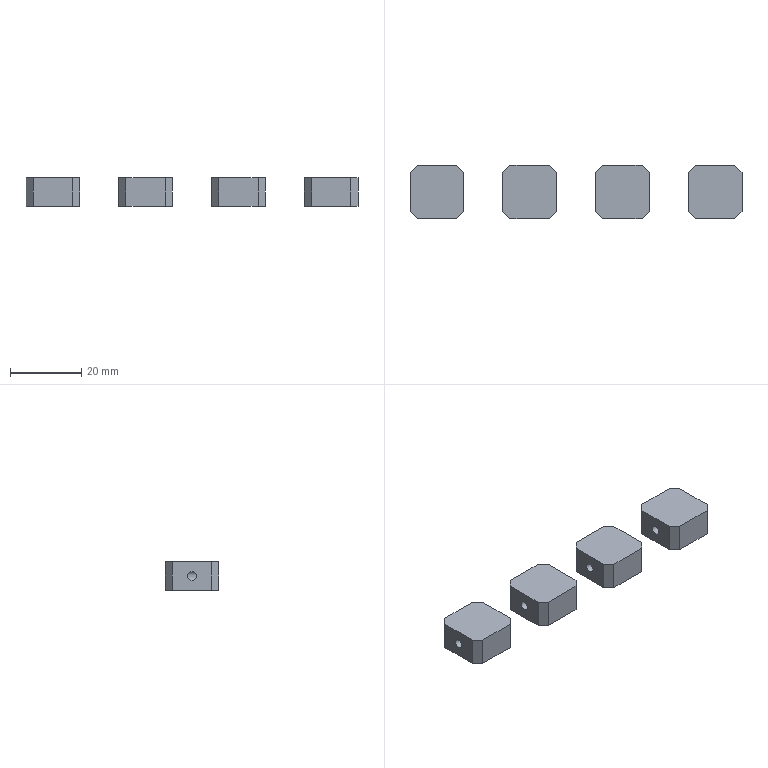Part | 4 solids | 52 faces | box 93 x 15 x 8 mm | volume 6470 mm3 | plane 40 | cylinder 8 | cone 4 | commonest cylinder face diameters 2.5 x4 3.3 x4
STEP:
#1=CARTESIAN_POINT('',(-5.5,7.5,8.));
#2=VERTEX_POINT('',#1);
#3=CARTESIAN_POINT('',(-7.5,5.5,8.));
#4=VERTEX_POINT('',#3);
#5=CARTESIAN_POINT('',(-6.5,6.5,8.));
#6=DIRECTION('',(-0.7071,-0.7071,0.));
#7=VECTOR('',#6,1000.);
#8=LINE('',#5,#7);
#9=EDGE_CURVE('',#2,#4,#8,.T.);
#10=ORIENTED_EDGE('',*,*,#9,.F.);
#11=CARTESIAN_POINT('',(-5.5,7.5,0.));
#12=VERTEX_POINT('',#11);
#13=CARTESIAN_POINT('',(-5.5,7.5,8.));
#14=DIRECTION('',(0.,0.,1.));
#15=VECTOR('',#14,1000.);
#16=LINE('',#13,#15);
#17=EDGE_CURVE('',#12,#2,#16,.T.);
#18=ORIENTED_EDGE('',*,*,#17,.F.);
#19=CARTESIAN_POINT('',(-7.5,5.5,0.));
#20=VERTEX_POINT('',#19);
#21=CARTESIAN_POINT('',(-7.5,5.5,0.));
#22=DIRECTION('',(0.7071,0.7071,0.));
#23=VECTOR('',#22,1000.);
#24=LINE('',#21,#23);
#25=EDGE_CURVE('',#20,#12,#24,.T.);
#26=ORIENTED_EDGE('',*,*,#25,.F.);
#27=CARTESIAN_POINT('',(-7.5,5.5,8.));
#28=DIRECTION('',(0.,0.,-1.));
#29=VECTOR('',#28,1000.);
#30=LINE('',#27,#29);
#31=EDGE_CURVE('',#4,#20,#30,.T.);
#32=ORIENTED_EDGE('',*,*,#31,.F.);
#33=EDGE_LOOP('',(#10,#18,#26,#32));
#34=FACE_BOUND('',#33,.T.);
#35=CARTESIAN_POINT('',(-7.5,5.5,8.));
#36=DIRECTION('',(0.7071,-0.7071,0.));
#37=DIRECTION('',(0.,0.,-1.));
#38=AXIS2_PLACEMENT_3D('',#35,#36,#37);
#39=PLANE('',#38);
#40=ADVANCED_FACE('',(#34),#39,.F.);
#41=CARTESIAN_POINT('',(-7.5,-5.5,8.));
#42=VERTEX_POINT('',#41);
#43=CARTESIAN_POINT('',(-5.5,-7.5,8.));
#44=VERTEX_POINT('',#43);
#45=CARTESIAN_POINT('',(-6.5,-6.5,8.));
#46=DIRECTION('',(0.7071,-0.7071,0.));
#47=VECTOR('',#46,1000.);
#48=LINE('',#45,#47);
#49=EDGE_CURVE('',#42,#44,#48,.T.);
#50=ORIENTED_EDGE('',*,*,#49,.F.);
#51=CARTESIAN_POINT('',(-7.5,-5.5,0.));
#52=VERTEX_POINT('',#51);
#53=CARTESIAN_POINT('',(-7.5,-5.5,8.));
#54=DIRECTION('',(0.,0.,1.));
#55=VECTOR('',#54,1000.);
#56=LINE('',#53,#55);
#57=EDGE_CURVE('',#52,#42,#56,.T.);
#58=ORIENTED_EDGE('',*,*,#57,.F.);
#59=CARTESIAN_POINT('',(-5.5,-7.5,0.));
#60=VERTEX_POINT('',#59);
#61=CARTESIAN_POINT('',(-5.5,-7.5,0.));
#62=DIRECTION('',(-0.7071,0.7071,0.));
#63=VECTOR('',#62,1000.);
#64=LINE('',#61,#63);
#65=EDGE_CURVE('',#60,#52,#64,.T.);
#66=ORIENTED_EDGE('',*,*,#65,.F.);
#67=CARTESIAN_POINT('',(-5.5,-7.5,8.));
#68=DIRECTION('',(0.,0.,-1.));
#69=VECTOR('',#68,1000.);
#70=LINE('',#67,#69);
#71=EDGE_CURVE('',#44,#60,#70,.T.);
#72=ORIENTED_EDGE('',*,*,#71,.F.);
#73=EDGE_LOOP('',(#50,#58,#66,#72));
#74=FACE_BOUND('',#73,.T.);
#75=CARTESIAN_POINT('',(-5.5,-7.5,8.));
#76=DIRECTION('',(0.7071,0.7071,0.));
#77=DIRECTION('',(0.,0.,-1.));
#78=AXIS2_PLACEMENT_3D('',#75,#76,#77);
#79=PLANE('',#78);
#80=ADVANCED_FACE('',(#74),#79,.F.);
#81=CARTESIAN_POINT('',(5.5,-7.5,8.));
#82=VERTEX_POINT('',#81);
#83=CARTESIAN_POINT('',(7.5,-5.5,8.));
#84=VERTEX_POINT('',#83);
#85=CARTESIAN_POINT('',(6.5,-6.5,8.));
#86=DIRECTION('',(0.7071,0.7071,0.));
#87=VECTOR('',#86,1000.);
#88=LINE('',#85,#87);
#89=EDGE_CURVE('',#82,#84,#88,.T.);
#90=ORIENTED_EDGE('',*,*,#89,.F.);
#91=CARTESIAN_POINT('',(5.5,-7.5,0.));
#92=VERTEX_POINT('',#91);
#93=CARTESIAN_POINT('',(5.5,-7.5,8.));
#94=DIRECTION('',(0.,0.,1.));
#95=VECTOR('',#94,1000.);
#96=LINE('',#93,#95);
#97=EDGE_CURVE('',#92,#82,#96,.T.);
#98=ORIENTED_EDGE('',*,*,#97,.F.);
#99=CARTESIAN_POINT('',(7.5,-5.5,0.));
#100=VERTEX_POINT('',#99);
#101=CARTESIAN_POINT('',(7.5,-5.5,0.));
#102=DIRECTION('',(-0.7071,-0.7071,0.));
#103=VECTOR('',#102,1000.);
#104=LINE('',#101,#103);
#105=EDGE_CURVE('',#100,#92,#104,.T.);
#106=ORIENTED_EDGE('',*,*,#105,.F.);
#107=CARTESIAN_POINT('',(7.5,-5.5,8.));
#108=DIRECTION('',(0.,0.,-1.));
#109=VECTOR('',#108,1000.);
#110=LINE('',#107,#109);
#111=EDGE_CURVE('',#84,#100,#110,.T.);
#112=ORIENTED_EDGE('',*,*,#111,.F.);
#113=EDGE_LOOP('',(#90,#98,#106,#112));
#114=FACE_BOUND('',#113,.T.);
#115=CARTESIAN_POINT('',(7.5,-5.5,8.));
#116=DIRECTION('',(-0.7071,0.7071,0.));
#117=DIRECTION('',(0.,0.,-1.));
#118=AXIS2_PLACEMENT_3D('',#115,#116,#117);
#119=PLANE('',#118);
#120=ADVANCED_FACE('',(#114),#119,.F.);
#121=CARTESIAN_POINT('',(7.5,5.5,8.));
#122=VERTEX_POINT('',#121);
#123=CARTESIAN_POINT('',(5.5,7.5,8.));
#124=VERTEX_POINT('',#123);
#125=CARTESIAN_POINT('',(6.5,6.5,8.));
#126=DIRECTION('',(-0.7071,0.7071,0.));
#127=VECTOR('',#126,1000.);
#128=LINE('',#125,#127);
#129=EDGE_CURVE('',#122,#124,#128,.T.);
#130=ORIENTED_EDGE('',*,*,#129,.F.);
#131=CARTESIAN_POINT('',(7.5,5.5,0.));
#132=VERTEX_POINT('',#131);
#133=CARTESIAN_POINT('',(7.5,5.5,8.));
#134=DIRECTION('',(0.,0.,1.));
#135=VECTOR('',#134,1000.);
#136=LINE('',#133,#135);
#137=EDGE_CURVE('',#132,#122,#136,.T.);
#138=ORIENTED_EDGE('',*,*,#137,.F.);
#139=CARTESIAN_POINT('',(5.5,7.5,0.));
#140=VERTEX_POINT('',#139);
#141=CARTESIAN_POINT('',(5.5,7.5,0.));
#142=DIRECTION('',(0.7071,-0.7071,0.));
#143=VECTOR('',#142,1000.);
#144=LINE('',#141,#143);
#145=EDGE_CURVE('',#140,#132,#144,.T.);
#146=ORIENTED_EDGE('',*,*,#145,.F.);
#147=CARTESIAN_POINT('',(5.5,7.5,8.));
#148=DIRECTION('',(0.,0.,-1.));
#149=VECTOR('',#148,1000.);
#150=LINE('',#147,#149);
#151=EDGE_CURVE('',#124,#140,#150,.T.);
#152=ORIENTED_EDGE('',*,*,#151,.F.);
#153=EDGE_LOOP('',(#130,#138,#146,#152));
#154=FACE_BOUND('',#153,.T.);
#155=CARTESIAN_POINT('',(5.5,7.5,8.));
#156=DIRECTION('',(-0.7071,-0.7071,0.));
#157=DIRECTION('',(0.,0.,-1.));
#158=AXIS2_PLACEMENT_3D('',#155,#156,#157);
#159=PLANE('',#158);
#160=ADVANCED_FACE('',(#154),#159,.F.);
#161=CARTESIAN_POINT('',(-7.5,7.5,0.));
#162=DIRECTION('',(-1.,0.,0.));
#163=VECTOR('',#162,1000.);
#164=LINE('',#161,#163);
#165=EDGE_CURVE('',#140,#12,#164,.T.);
#166=ORIENTED_EDGE('',*,*,#165,.F.);
#167=ORIENTED_EDGE('',*,*,#145,.T.);
#168=CARTESIAN_POINT('',(7.5,7.5,0.));
#169=DIRECTION('',(0.,1.,0.));
#170=VECTOR('',#169,1000.);
#171=LINE('',#168,#170);
#172=EDGE_CURVE('',#100,#132,#171,.T.);
#173=ORIENTED_EDGE('',*,*,#172,.F.);
#174=ORIENTED_EDGE('',*,*,#105,.T.);
#175=CARTESIAN_POINT('',(-7.5,-7.5,0.));
#176=DIRECTION('',(1.,0.,0.));
#177=VECTOR('',#176,1000.);
#178=LINE('',#175,#177);
#179=EDGE_CURVE('',#60,#92,#178,.T.);
#180=ORIENTED_EDGE('',*,*,#179,.F.);
#181=ORIENTED_EDGE('',*,*,#65,.T.);
#182=CARTESIAN_POINT('',(-7.5,7.5,0.));
#183=DIRECTION('',(0.,-1.,0.));
#184=VECTOR('',#183,1000.);
#185=LINE('',#182,#184);
#186=EDGE_CURVE('',#20,#52,#185,.T.);
#187=ORIENTED_EDGE('',*,*,#186,.F.);
#188=ORIENTED_EDGE('',*,*,#25,.T.);
#189=EDGE_LOOP('',(#166,#167,#173,#174,#180,#181,#187,#188));
#190=FACE_BOUND('',#189,.T.);
#191=CARTESIAN_POINT('',(0.,0.,0.));
#192=DIRECTION('',(0.,0.,1.));
#193=DIRECTION('',(1.,0.,0.));
#194=AXIS2_PLACEMENT_3D('',#191,#192,#193);
#195=PLANE('',#194);
#196=ADVANCED_FACE('',(#190),#195,.F.);
#197=CARTESIAN_POINT('',(7.5,7.5,8.));
#198=DIRECTION('',(0.,1.,0.));
#199=VECTOR('',#198,1000.);
#200=LINE('',#197,#199);
#201=EDGE_CURVE('',#84,#122,#200,.T.);
#202=ORIENTED_EDGE('',*,*,#201,.T.);
#203=ORIENTED_EDGE('',*,*,#129,.T.);
#204=CARTESIAN_POINT('',(-7.5,7.5,8.));
#205=DIRECTION('',(-1.,0.,0.));
#206=VECTOR('',#205,1000.);
#207=LINE('',#204,#206);
#208=EDGE_CURVE('',#124,#2,#207,.T.);
#209=ORIENTED_EDGE('',*,*,#208,.T.);
#210=ORIENTED_EDGE('',*,*,#9,.T.);
#211=CARTESIAN_POINT('',(-7.5,7.5,8.));
#212=DIRECTION('',(0.,-1.,0.));
#213=VECTOR('',#212,1000.);
#214=LINE('',#211,#213);
#215=EDGE_CURVE('',#4,#42,#214,.T.);
#216=ORIENTED_EDGE('',*,*,#215,.T.);
#217=ORIENTED_EDGE('',*,*,#49,.T.);
#218=CARTESIAN_POINT('',(-7.5,-7.5,8.));
#219=DIRECTION('',(1.,0.,0.));
#220=VECTOR('',#219,1000.);
#221=LINE('',#218,#220);
#222=EDGE_CURVE('',#44,#82,#221,.T.);
#223=ORIENTED_EDGE('',*,*,#222,.T.);
#224=ORIENTED_EDGE('',*,*,#89,.T.);
#225=EDGE_LOOP('',(#202,#203,#209,#210,#216,#217,#223,#224));
#226=FACE_BOUND('',#225,.T.);
#227=CARTESIAN_POINT('',(0.,0.,8.));
#228=DIRECTION('',(0.,0.,1.));
#229=DIRECTION('',(1.,0.,0.));
#230=AXIS2_PLACEMENT_3D('',#227,#228,#229);
#231=PLANE('',#230);
#232=ADVANCED_FACE('',(#226),#231,.T.);
#233=ORIENTED_EDGE('',*,*,#179,.T.);
#234=ORIENTED_EDGE('',*,*,#97,.T.);
#235=ORIENTED_EDGE('',*,*,#222,.F.);
#236=ORIENTED_EDGE('',*,*,#71,.T.);
#237=EDGE_LOOP('',(#233,#234,#235,#236));
#238=FACE_BOUND('',#237,.T.);
#239=CARTESIAN_POINT('',(-7.5,-7.5,8.));
#240=DIRECTION('',(0.,1.,0.));
#241=DIRECTION('',(0.,0.,1.));
#242=AXIS2_PLACEMENT_3D('',#239,#240,#241);
#243=PLANE('',#242);
#244=ADVANCED_FACE('',(#238),#243,.F.);
#245=ORIENTED_EDGE('',*,*,#186,.T.);
#246=ORIENTED_EDGE('',*,*,#57,.T.);
#247=ORIENTED_EDGE('',*,*,#215,.F.);
#248=ORIENTED_EDGE('',*,*,#31,.T.);
#249=EDGE_LOOP('',(#245,#246,#247,#248));
#250=FACE_BOUND('',#249,.T.);
#251=CARTESIAN_POINT('',(-7.5,0.,5.25));
#252=VERTEX_POINT('',#251);
#253=CARTESIAN_POINT('',(-7.5,0.,4.));
#254=DIRECTION('',(-1.,0.,0.));
#255=DIRECTION('',(0.,0.,1.));
#256=AXIS2_PLACEMENT_3D('',#253,#254,#255);
#257=CIRCLE('',#256,1.25);
#258=EDGE_CURVE('',#252,#252,#257,.T.);
#259=ORIENTED_EDGE('',*,*,#258,.F.);
#260=EDGE_LOOP('',(#259));
#261=FACE_BOUND('',#260,.T.);
#262=CARTESIAN_POINT('',(-7.5,7.5,8.));
#263=DIRECTION('',(1.,0.,0.));
#264=DIRECTION('',(0.,1.,0.));
#265=AXIS2_PLACEMENT_3D('',#262,#263,#264);
#266=PLANE('',#265);
#267=ADVANCED_FACE('',(#250,#261),#266,.F.);
#268=ORIENTED_EDGE('',*,*,#208,.F.);
#269=ORIENTED_EDGE('',*,*,#151,.T.);
#270=ORIENTED_EDGE('',*,*,#165,.T.);
#271=ORIENTED_EDGE('',*,*,#17,.T.);
#272=EDGE_LOOP('',(#268,#269,#270,#271));
#273=FACE_BOUND('',#272,.T.);
#274=CARTESIAN_POINT('',(0.,7.5,5.65));
#275=VERTEX_POINT('',#274);
#276=CARTESIAN_POINT('',(0.,7.5,4.));
#277=DIRECTION('',(0.,1.,0.));
#278=DIRECTION('',(0.,0.,1.));
#279=AXIS2_PLACEMENT_3D('',#276,#277,#278);
#280=CIRCLE('',#279,1.65);
#281=EDGE_CURVE('',#275,#275,#280,.T.);
#282=ORIENTED_EDGE('',*,*,#281,.F.);
#283=EDGE_LOOP('',(#282));
#284=FACE_BOUND('',#283,.T.);
#285=CARTESIAN_POINT('',(-7.5,7.5,8.));
#286=DIRECTION('',(0.,-1.,0.));
#287=DIRECTION('',(0.,0.,-1.));
#288=AXIS2_PLACEMENT_3D('',#285,#286,#287);
#289=PLANE('',#288);
#290=ADVANCED_FACE('',(#273,#284),#289,.F.);
#291=ORIENTED_EDGE('',*,*,#172,.T.);
#292=ORIENTED_EDGE('',*,*,#137,.T.);
#293=ORIENTED_EDGE('',*,*,#201,.F.);
#294=ORIENTED_EDGE('',*,*,#111,.T.);
#295=EDGE_LOOP('',(#291,#292,#293,#294));
#296=FACE_BOUND('',#295,.T.);
#297=CARTESIAN_POINT('',(7.5,7.5,8.));
#298=DIRECTION('',(-1.,0.,0.));
#299=DIRECTION('',(0.,-1.,0.));
#300=AXIS2_PLACEMENT_3D('',#297,#298,#299);
#301=PLANE('',#300);
#302=ADVANCED_FACE('',(#296),#301,.F.);
#303=CARTESIAN_POINT('',(0.,-2.6,5.65));
#304=VERTEX_POINT('',#303);
#305=CARTESIAN_POINT('',(0.,-2.6,4.));
#306=DIRECTION('',(0.,1.,0.));
#307=DIRECTION('',(0.,0.,1.));
#308=AXIS2_PLACEMENT_3D('',#305,#306,#307);
#309=CIRCLE('',#308,1.65);
#310=EDGE_CURVE('',#304,#304,#309,.T.);
#311=ORIENTED_EDGE('',*,*,#310,.T.);
#312=EDGE_LOOP('',(#311));
#313=FACE_BOUND('',#312,.T.);
#314=CARTESIAN_POINT('',(0.,-3.591,4.));
#315=VERTEX_POINT('',#314);
#316=VERTEX_LOOP('',#315);
#317=FACE_BOUND('',#316,.T.);
#318=CARTESIAN_POINT('',(0.,-2.6,4.));
#319=DIRECTION('',(0.,1.,0.));
#320=DIRECTION('',(0.,0.,1.));
#321=AXIS2_PLACEMENT_3D('',#318,#319,#320);
#322=CONICAL_SURFACE('',#321,1.65,1.03);
#323=ADVANCED_FACE('',(#313,#317),#322,.F.);
#324=ORIENTED_EDGE('',*,*,#310,.F.);
#325=EDGE_LOOP('',(#324));
#326=FACE_BOUND('',#325,.T.);
#327=ORIENTED_EDGE('',*,*,#281,.T.);
#328=EDGE_LOOP('',(#327));
#329=FACE_BOUND('',#328,.T.);
#330=CARTESIAN_POINT('',(-1.077,0.,2.75));
#331=VERTEX_POINT('',#330);
#332=CARTESIAN_POINT('',(-1.417,0.9718,3.012));
#333=CARTESIAN_POINT('',(-0.9074,-0.0006623,2.619));
#334=CARTESIAN_POINT('',(-1.416,-0.9692,3.011));
#335=CARTESIAN_POINT('',(-1.767,-1.39,3.997));
#336=CARTESIAN_POINT('',(-1.416,-0.9715,4.989));
#337=CARTESIAN_POINT('',(-0.9074,0.00335,5.381));
#338=CARTESIAN_POINT('',(-1.416,0.9694,4.988));
#339=CARTESIAN_POINT('',(-1.767,1.39,4.003));
#340=CARTESIAN_POINT('',(-1.417,0.9718,3.012));
#341=CARTESIAN_POINT('',(-0.9074,-0.0006623,2.619));
#342=CARTESIAN_POINT('',(-1.416,-0.9692,3.011));
#343=B_SPLINE_CURVE_WITH_KNOTS('',3,(#332,#333,#334,#335,#336,#337,#338,#339,#340,#341,#342),.UNSPECIFIED.,.T.,.F.,(1,1,1,1,1,1,1,1,1,1,1,1,1,1,1),(-0.003071,-0.002047,-0.001024,0.,0.001024,0.002047,0.003071,0.004095,0.005119,0.006142,0.007166,0.00819,0.009214,0.01024,0.01126),.UNSPECIFIED.);
#344=EDGE_CURVE('',#331,#331,#343,.T.);
#345=ORIENTED_EDGE('',*,*,#344,.T.);
#346=EDGE_LOOP('',(#345));
#347=FACE_BOUND('',#346,.T.);
#348=CARTESIAN_POINT('',(0.,7.5,4.));
#349=DIRECTION('',(0.,1.,0.));
#350=DIRECTION('',(0.,0.,1.));
#351=AXIS2_PLACEMENT_3D('',#348,#349,#350);
#352=CYLINDRICAL_SURFACE('',#351,1.65);
#353=ADVANCED_FACE('',(#326,#329,#347),#352,.F.);
#354=ORIENTED_EDGE('',*,*,#344,.F.);
#355=EDGE_LOOP('',(#354));
#356=FACE_BOUND('',#355,.T.);
#357=ORIENTED_EDGE('',*,*,#258,.T.);
#358=EDGE_LOOP('',(#357));
#359=FACE_BOUND('',#358,.T.);
#360=CARTESIAN_POINT('',(-7.5,0.,4.));
#361=DIRECTION('',(-1.,0.,0.));
#362=DIRECTION('',(0.,0.,1.));
#363=AXIS2_PLACEMENT_3D('',#360,#361,#362);
#364=CYLINDRICAL_SURFACE('',#363,1.25);
#365=ADVANCED_FACE('',(#356,#359),#364,.F.);
#366=CLOSED_SHELL('',(#40,#80,#120,#160,#196,#232,#244,#267,#290,#302,#323,#353,#365));
#367=MANIFOLD_SOLID_BREP('',#366);
#368=CARTESIAN_POINT('',(20.5,7.5,8.));
#369=VERTEX_POINT('',#368);
#370=CARTESIAN_POINT('',(18.5,5.5,8.));
#371=VERTEX_POINT('',#370);
#372=CARTESIAN_POINT('',(19.5,6.5,8.));
#373=DIRECTION('',(-0.7071,-0.7071,0.));
#374=VECTOR('',#373,1000.);
#375=LINE('',#372,#374);
#376=EDGE_CURVE('',#369,#371,#375,.T.);
#377=ORIENTED_EDGE('',*,*,#376,.F.);
#378=CARTESIAN_POINT('',(20.5,7.5,0.));
#379=VERTEX_POINT('',#378);
#380=CARTESIAN_POINT('',(20.5,7.5,8.));
#381=DIRECTION('',(0.,0.,1.));
#382=VECTOR('',#381,1000.);
#383=LINE('',#380,#382);
#384=EDGE_CURVE('',#379,#369,#383,.T.);
#385=ORIENTED_EDGE('',*,*,#384,.F.);
#386=CARTESIAN_POINT('',(18.5,5.5,0.));
#387=VERTEX_POINT('',#386);
#388=CARTESIAN_POINT('',(18.5,5.5,0.));
#389=DIRECTION('',(0.7071,0.7071,0.));
#390=VECTOR('',#389,1000.);
#391=LINE('',#388,#390);
#392=EDGE_CURVE('',#387,#379,#391,.T.);
#393=ORIENTED_EDGE('',*,*,#392,.F.);
#394=CARTESIAN_POINT('',(18.5,5.5,8.));
#395=DIRECTION('',(0.,0.,-1.));
#396=VECTOR('',#395,1000.);
#397=LINE('',#394,#396);
#398=EDGE_CURVE('',#371,#387,#397,.T.);
#399=ORIENTED_EDGE('',*,*,#398,.F.);
#400=EDGE_LOOP('',(#377,#385,#393,#399));
#401=FACE_BOUND('',#400,.T.);
#402=CARTESIAN_POINT('',(18.5,5.5,8.));
#403=DIRECTION('',(0.7071,-0.7071,0.));
#404=DIRECTION('',(0.,0.,-1.));
#405=AXIS2_PLACEMENT_3D('',#402,#403,#404);
#406=PLANE('',#405);
#407=ADVANCED_FACE('',(#401),#406,.F.);
#408=CARTESIAN_POINT('',(18.5,-5.5,8.));
#409=VERTEX_POINT('',#408);
#410=CARTESIAN_POINT('',(20.5,-7.5,8.));
#411=VERTEX_POINT('',#410);
#412=CARTESIAN_POINT('',(19.5,-6.5,8.));
#413=DIRECTION('',(0.7071,-0.7071,0.));
#414=VECTOR('',#413,1000.);
#415=LINE('',#412,#414);
#416=EDGE_CURVE('',#409,#411,#415,.T.);
#417=ORIENTED_EDGE('',*,*,#416,.F.);
#418=CARTESIAN_POINT('',(18.5,-5.5,0.));
#419=VERTEX_POINT('',#418);
#420=CARTESIAN_POINT('',(18.5,-5.5,8.));
#421=DIRECTION('',(0.,0.,1.));
#422=VECTOR('',#421,1000.);
#423=LINE('',#420,#422);
#424=EDGE_CURVE('',#419,#409,#423,.T.);
#425=ORIENTED_EDGE('',*,*,#424,.F.);
#426=CARTESIAN_POINT('',(20.5,-7.5,0.));
#427=VERTEX_POINT('',#426);
#428=CARTESIAN_POINT('',(20.5,-7.5,0.));
#429=DIRECTION('',(-0.7071,0.7071,0.));
#430=VECTOR('',#429,1000.);
#431=LINE('',#428,#430);
#432=EDGE_CURVE('',#427,#419,#431,.T.);
#433=ORIENTED_EDGE('',*,*,#432,.F.);
#434=CARTESIAN_POINT('',(20.5,-7.5,8.));
#435=DIRECTION('',(0.,0.,-1.));
#436=VECTOR('',#435,1000.);
#437=LINE('',#434,#436);
#438=EDGE_CURVE('',#411,#427,#437,.T.);
#439=ORIENTED_EDGE('',*,*,#438,.F.);
#440=EDGE_LOOP('',(#417,#425,#433,#439));
#441=FACE_BOUND('',#440,.T.);
#442=CARTESIAN_POINT('',(20.5,-7.5,8.));
#443=DIRECTION('',(0.7071,0.7071,0.));
#444=DIRECTION('',(0.,0.,-1.));
#445=AXIS2_PLACEMENT_3D('',#442,#443,#444);
#446=PLANE('',#445);
#447=ADVANCED_FACE('',(#441),#446,.F.);
#448=CARTESIAN_POINT('',(31.5,-7.5,8.));
#449=VERTEX_POINT('',#448);
#450=CARTESIAN_POINT('',(33.5,-5.5,8.));
#451=VERTEX_POINT('',#450);
#452=CARTESIAN_POINT('',(32.5,-6.5,8.));
#453=DIRECTION('',(0.7071,0.7071,0.));
#454=VECTOR('',#453,1000.);
#455=LINE('',#452,#454);
#456=EDGE_CURVE('',#449,#451,#455,.T.);
#457=ORIENTED_EDGE('',*,*,#456,.F.);
#458=CARTESIAN_POINT('',(31.5,-7.5,0.));
#459=VERTEX_POINT('',#458);
#460=CARTESIAN_POINT('',(31.5,-7.5,8.));
#461=DIRECTION('',(0.,0.,1.));
#462=VECTOR('',#461,1000.);
#463=LINE('',#460,#462);
#464=EDGE_CURVE('',#459,#449,#463,.T.);
#465=ORIENTED_EDGE('',*,*,#464,.F.);
#466=CARTESIAN_POINT('',(33.5,-5.5,0.));
#467=VERTEX_POINT('',#466);
#468=CARTESIAN_POINT('',(33.5,-5.5,0.));
#469=DIRECTION('',(-0.7071,-0.7071,0.));
#470=VECTOR('',#469,1000.);
#471=LINE('',#468,#470);
#472=EDGE_CURVE('',#467,#459,#471,.T.);
#473=ORIENTED_EDGE('',*,*,#472,.F.);
#474=CARTESIAN_POINT('',(33.5,-5.5,8.));
#475=DIRECTION('',(0.,0.,-1.));
#476=VECTOR('',#475,1000.);
#477=LINE('',#474,#476);
#478=EDGE_CURVE('',#451,#467,#477,.T.);
#479=ORIENTED_EDGE('',*,*,#478,.F.);
#480=EDGE_LOOP('',(#457,#465,#473,#479));
#481=FACE_BOUND('',#480,.T.);
#482=CARTESIAN_POINT('',(33.5,-5.5,8.));
#483=DIRECTION('',(-0.7071,0.7071,0.));
#484=DIRECTION('',(0.,0.,-1.));
#485=AXIS2_PLACEMENT_3D('',#482,#483,#484);
#486=PLANE('',#485);
#487=ADVANCED_FACE('',(#481),#486,.F.);
#488=CARTESIAN_POINT('',(33.5,5.5,8.));
#489=VERTEX_POINT('',#488);
#490=CARTESIAN_POINT('',(31.5,7.5,8.));
#491=VERTEX_POINT('',#490);
#492=CARTESIAN_POINT('',(32.5,6.5,8.));
#493=DIRECTION('',(-0.7071,0.7071,0.));
#494=VECTOR('',#493,1000.);
#495=LINE('',#492,#494);
#496=EDGE_CURVE('',#489,#491,#495,.T.);
#497=ORIENTED_EDGE('',*,*,#496,.F.);
#498=CARTESIAN_POINT('',(33.5,5.5,0.));
#499=VERTEX_POINT('',#498);
#500=CARTESIAN_POINT('',(33.5,5.5,8.));
#501=DIRECTION('',(0.,0.,1.));
#502=VECTOR('',#501,1000.);
#503=LINE('',#500,#502);
#504=EDGE_CURVE('',#499,#489,#503,.T.);
#505=ORIENTED_EDGE('',*,*,#504,.F.);
#506=CARTESIAN_POINT('',(31.5,7.5,0.));
#507=VERTEX_POINT('',#506);
#508=CARTESIAN_POINT('',(31.5,7.5,0.));
#509=DIRECTION('',(0.7071,-0.7071,0.));
#510=VECTOR('',#509,1000.);
#511=LINE('',#508,#510);
#512=EDGE_CURVE('',#507,#499,#511,.T.);
#513=ORIENTED_EDGE('',*,*,#512,.F.);
#514=CARTESIAN_POINT('',(31.5,7.5,8.));
#515=DIRECTION('',(0.,0.,-1.));
#516=VECTOR('',#515,1000.);
#517=LINE('',#514,#516);
#518=EDGE_CURVE('',#491,#507,#517,.T.);
#519=ORIENTED_EDGE('',*,*,#518,.F.);
#520=EDGE_LOOP('',(#497,#505,#513,#519));
#521=FACE_BOUND('',#520,.T.);
#522=CARTESIAN_POINT('',(31.5,7.5,8.));
#523=DIRECTION('',(-0.7071,-0.7071,0.));
#524=DIRECTION('',(0.,0.,-1.));
#525=AXIS2_PLACEMENT_3D('',#522,#523,#524);
#526=PLANE('',#525);
#527=ADVANCED_FACE('',(#521),#526,.F.);
#528=CARTESIAN_POINT('',(18.5,7.5,0.));
#529=DIRECTION('',(-1.,0.,0.));
#530=VECTOR('',#529,1000.);
#531=LINE('',#528,#530);
#532=EDGE_CURVE('',#507,#379,#531,.T.);
#533=ORIENTED_EDGE('',*,*,#532,.F.);
#534=ORIENTED_EDGE('',*,*,#512,.T.);
#535=CARTESIAN_POINT('',(33.5,7.5,0.));
#536=DIRECTION('',(0.,1.,0.));
#537=VECTOR('',#536,1000.);
#538=LINE('',#535,#537);
#539=EDGE_CURVE('',#467,#499,#538,.T.);
#540=ORIENTED_EDGE('',*,*,#539,.F.);
#541=ORIENTED_EDGE('',*,*,#472,.T.);
#542=CARTESIAN_POINT('',(18.5,-7.5,0.));
#543=DIRECTION('',(1.,0.,0.));
#544=VECTOR('',#543,1000.);
#545=LINE('',#542,#544);
#546=EDGE_CURVE('',#427,#459,#545,.T.);
#547=ORIENTED_EDGE('',*,*,#546,.F.);
#548=ORIENTED_EDGE('',*,*,#432,.T.);
#549=CARTESIAN_POINT('',(18.5,7.5,0.));
#550=DIRECTION('',(0.,-1.,0.));
#551=VECTOR('',#550,1000.);
#552=LINE('',#549,#551);
#553=EDGE_CURVE('',#387,#419,#552,.T.);
#554=ORIENTED_EDGE('',*,*,#553,.F.);
#555=ORIENTED_EDGE('',*,*,#392,.T.);
#556=EDGE_LOOP('',(#533,#534,#540,#541,#547,#548,#554,#555));
#557=FACE_BOUND('',#556,.T.);
#558=CARTESIAN_POINT('',(26.,0.,0.));
#559=DIRECTION('',(0.,0.,1.));
#560=DIRECTION('',(1.,0.,0.));
#561=AXIS2_PLACEMENT_3D('',#558,#559,#560);
#562=PLANE('',#561);
#563=ADVANCED_FACE('',(#557),#562,.F.);
#564=CARTESIAN_POINT('',(33.5,7.5,8.));
#565=DIRECTION('',(0.,1.,0.));
#566=VECTOR('',#565,1000.);
#567=LINE('',#564,#566);
#568=EDGE_CURVE('',#451,#489,#567,.T.);
#569=ORIENTED_EDGE('',*,*,#568,.T.);
#570=ORIENTED_EDGE('',*,*,#496,.T.);
#571=CARTESIAN_POINT('',(18.5,7.5,8.));
#572=DIRECTION('',(-1.,0.,0.));
#573=VECTOR('',#572,1000.);
#574=LINE('',#571,#573);
#575=EDGE_CURVE('',#491,#369,#574,.T.);
#576=ORIENTED_EDGE('',*,*,#575,.T.);
#577=ORIENTED_EDGE('',*,*,#376,.T.);
#578=CARTESIAN_POINT('',(18.5,7.5,8.));
#579=DIRECTION('',(0.,-1.,0.));
#580=VECTOR('',#579,1000.);
#581=LINE('',#578,#580);
#582=EDGE_CURVE('',#371,#409,#581,.T.);
#583=ORIENTED_EDGE('',*,*,#582,.T.);
#584=ORIENTED_EDGE('',*,*,#416,.T.);
#585=CARTESIAN_POINT('',(18.5,-7.5,8.));
#586=DIRECTION('',(1.,0.,0.));
#587=VECTOR('',#586,1000.);
#588=LINE('',#585,#587);
#589=EDGE_CURVE('',#411,#449,#588,.T.);
#590=ORIENTED_EDGE('',*,*,#589,.T.);
#591=ORIENTED_EDGE('',*,*,#456,.T.);
#592=EDGE_LOOP('',(#569,#570,#576,#577,#583,#584,#590,#591));
#593=FACE_BOUND('',#592,.T.);
#594=CARTESIAN_POINT('',(26.,0.,8.));
#595=DIRECTION('',(0.,0.,1.));
#596=DIRECTION('',(1.,0.,0.));
#597=AXIS2_PLACEMENT_3D('',#594,#595,#596);
#598=PLANE('',#597);
#599=ADVANCED_FACE('',(#593),#598,.T.);
#600=ORIENTED_EDGE('',*,*,#546,.T.);
#601=ORIENTED_EDGE('',*,*,#464,.T.);
#602=ORIENTED_EDGE('',*,*,#589,.F.);
#603=ORIENTED_EDGE('',*,*,#438,.T.);
#604=EDGE_LOOP('',(#600,#601,#602,#603));
#605=FACE_BOUND('',#604,.T.);
#606=CARTESIAN_POINT('',(18.5,-7.5,8.));
#607=DIRECTION('',(0.,1.,0.));
#608=DIRECTION('',(0.,0.,1.));
#609=AXIS2_PLACEMENT_3D('',#606,#607,#608);
#610=PLANE('',#609);
#611=ADVANCED_FACE('',(#605),#610,.F.);
#612=ORIENTED_EDGE('',*,*,#553,.T.);
#613=ORIENTED_EDGE('',*,*,#424,.T.);
#614=ORIENTED_EDGE('',*,*,#582,.F.);
#615=ORIENTED_EDGE('',*,*,#398,.T.);
#616=EDGE_LOOP('',(#612,#613,#614,#615));
#617=FACE_BOUND('',#616,.T.);
#618=CARTESIAN_POINT('',(18.5,0.,5.25));
#619=VERTEX_POINT('',#618);
#620=CARTESIAN_POINT('',(18.5,0.,4.));
#621=DIRECTION('',(-1.,0.,0.));
#622=DIRECTION('',(0.,0.,1.));
#623=AXIS2_PLACEMENT_3D('',#620,#621,#622);
#624=CIRCLE('',#623,1.25);
#625=EDGE_CURVE('',#619,#619,#624,.T.);
#626=ORIENTED_EDGE('',*,*,#625,.F.);
#627=EDGE_LOOP('',(#626));
#628=FACE_BOUND('',#627,.T.);
#629=CARTESIAN_POINT('',(18.5,7.5,8.));
#630=DIRECTION('',(1.,0.,0.));
#631=DIRECTION('',(0.,1.,0.));
#632=AXIS2_PLACEMENT_3D('',#629,#630,#631);
#633=PLANE('',#632);
#634=ADVANCED_FACE('',(#617,#628),#633,.F.);
#635=ORIENTED_EDGE('',*,*,#575,.F.);
#636=ORIENTED_EDGE('',*,*,#518,.T.);
#637=ORIENTED_EDGE('',*,*,#532,.T.);
#638=ORIENTED_EDGE('',*,*,#384,.T.);
#639=EDGE_LOOP('',(#635,#636,#637,#638));
#640=FACE_BOUND('',#639,.T.);
#641=CARTESIAN_POINT('',(26.,7.5,5.65));
#642=VERTEX_POINT('',#641);
#643=CARTESIAN_POINT('',(26.,7.5,4.));
#644=DIRECTION('',(0.,1.,0.));
#645=DIRECTION('',(0.,0.,1.));
#646=AXIS2_PLACEMENT_3D('',#643,#644,#645);
#647=CIRCLE('',#646,1.65);
#648=EDGE_CURVE('',#642,#642,#647,.T.);
#649=ORIENTED_EDGE('',*,*,#648,.F.);
#650=EDGE_LOOP('',(#649));
#651=FACE_BOUND('',#650,.T.);
#652=CARTESIAN_POINT('',(18.5,7.5,8.));
#653=DIRECTION('',(0.,-1.,0.));
#654=DIRECTION('',(0.,0.,-1.));
#655=AXIS2_PLACEMENT_3D('',#652,#653,#654);
#656=PLANE('',#655);
#657=ADVANCED_FACE('',(#640,#651),#656,.F.);
#658=ORIENTED_EDGE('',*,*,#539,.T.);
#659=ORIENTED_EDGE('',*,*,#504,.T.);
#660=ORIENTED_EDGE('',*,*,#568,.F.);
#661=ORIENTED_EDGE('',*,*,#478,.T.);
#662=EDGE_LOOP('',(#658,#659,#660,#661));
#663=FACE_BOUND('',#662,.T.);
#664=CARTESIAN_POINT('',(33.5,7.5,8.));
#665=DIRECTION('',(-1.,0.,0.));
#666=DIRECTION('',(0.,-1.,0.));
#667=AXIS2_PLACEMENT_3D('',#664,#665,#666);
#668=PLANE('',#667);
#669=ADVANCED_FACE('',(#663),#668,.F.);
#670=CARTESIAN_POINT('',(26.,-2.6,5.65));
#671=VERTEX_POINT('',#670);
#672=CARTESIAN_POINT('',(26.,-2.6,4.));
#673=DIRECTION('',(0.,1.,0.));
#674=DIRECTION('',(0.,0.,1.));
#675=AXIS2_PLACEMENT_3D('',#672,#673,#674);
#676=CIRCLE('',#675,1.65);
#677=EDGE_CURVE('',#671,#671,#676,.T.);
#678=ORIENTED_EDGE('',*,*,#677,.T.);
#679=EDGE_LOOP('',(#678));
#680=FACE_BOUND('',#679,.T.);
#681=CARTESIAN_POINT('',(26.,-3.591,4.));
#682=VERTEX_POINT('',#681);
#683=VERTEX_LOOP('',#682);
#684=FACE_BOUND('',#683,.T.);
#685=CARTESIAN_POINT('',(26.,-2.6,4.));
#686=DIRECTION('',(0.,1.,0.));
#687=DIRECTION('',(0.,0.,1.));
#688=AXIS2_PLACEMENT_3D('',#685,#686,#687);
#689=CONICAL_SURFACE('',#688,1.65,1.03);
#690=ADVANCED_FACE('',(#680,#684),#689,.F.);
#691=ORIENTED_EDGE('',*,*,#677,.F.);
#692=EDGE_LOOP('',(#691));
#693=FACE_BOUND('',#692,.T.);
#694=ORIENTED_EDGE('',*,*,#648,.T.);
#695=EDGE_LOOP('',(#694));
#696=FACE_BOUND('',#695,.T.);
#697=CARTESIAN_POINT('',(24.923,0.,2.75));
#698=VERTEX_POINT('',#697);
#699=CARTESIAN_POINT('',(24.583,0.9718,3.012));
#700=CARTESIAN_POINT('',(25.093,-0.0006623,2.619));
#701=CARTESIAN_POINT('',(24.584,-0.9692,3.011));
#702=CARTESIAN_POINT('',(24.233,-1.39,3.997));
#703=CARTESIAN_POINT('',(24.584,-0.9715,4.989));
#704=CARTESIAN_POINT('',(25.093,0.00335,5.381));
#705=CARTESIAN_POINT('',(24.584,0.9694,4.988));
#706=CARTESIAN_POINT('',(24.233,1.39,4.003));
#707=CARTESIAN_POINT('',(24.583,0.9718,3.012));
#708=CARTESIAN_POINT('',(25.093,-0.0006623,2.619));
#709=CARTESIAN_POINT('',(24.584,-0.9692,3.011));
#710=B_SPLINE_CURVE_WITH_KNOTS('',3,(#699,#700,#701,#702,#703,#704,#705,#706,#707,#708,#709),.UNSPECIFIED.,.T.,.F.,(1,1,1,1,1,1,1,1,1,1,1,1,1,1,1),(-0.003071,-0.002047,-0.001024,0.,0.001024,0.002047,0.003071,0.004095,0.005119,0.006142,0.007166,0.00819,0.009214,0.01024,0.01126),.UNSPECIFIED.);
#711=EDGE_CURVE('',#698,#698,#710,.T.);
#712=ORIENTED_EDGE('',*,*,#711,.T.);
#713=EDGE_LOOP('',(#712));
#714=FACE_BOUND('',#713,.T.);
#715=CARTESIAN_POINT('',(26.,7.5,4.));
#716=DIRECTION('',(0.,1.,0.));
#717=DIRECTION('',(0.,0.,1.));
#718=AXIS2_PLACEMENT_3D('',#715,#716,#717);
#719=CYLINDRICAL_SURFACE('',#718,1.65);
#720=ADVANCED_FACE('',(#693,#696,#714),#719,.F.);
#721=ORIENTED_EDGE('',*,*,#711,.F.);
#722=EDGE_LOOP('',(#721));
#723=FACE_BOUND('',#722,.T.);
#724=ORIENTED_EDGE('',*,*,#625,.T.);
#725=EDGE_LOOP('',(#724));
#726=FACE_BOUND('',#725,.T.);
#727=CARTESIAN_POINT('',(18.5,0.,4.));
#728=DIRECTION('',(-1.,0.,0.));
#729=DIRECTION('',(0.,0.,1.));
#730=AXIS2_PLACEMENT_3D('',#727,#728,#729);
#731=CYLINDRICAL_SURFACE('',#730,1.25);
#732=ADVANCED_FACE('',(#723,#726),#731,.F.);
#733=CLOSED_SHELL('',(#407,#447,#487,#527,#563,#599,#611,#634,#657,#669,#690,#720,#732));
#734=MANIFOLD_SOLID_BREP('',#733);
#735=CARTESIAN_POINT('',(72.5,7.5,8.));
#736=VERTEX_POINT('',#735);
#737=CARTESIAN_POINT('',(70.5,5.5,8.));
#738=VERTEX_POINT('',#737);
#739=CARTESIAN_POINT('',(71.5,6.5,8.));
#740=DIRECTION('',(-0.7071,-0.7071,0.));
#741=VECTOR('',#740,1000.);
#742=LINE('',#739,#741);
#743=EDGE_CURVE('',#736,#738,#742,.T.);
#744=ORIENTED_EDGE('',*,*,#743,.F.);
#745=CARTESIAN_POINT('',(72.5,7.5,0.));
#746=VERTEX_POINT('',#745);
#747=CARTESIAN_POINT('',(72.5,7.5,8.));
#748=DIRECTION('',(0.,0.,1.));
#749=VECTOR('',#748,1000.);
#750=LINE('',#747,#749);
#751=EDGE_CURVE('',#746,#736,#750,.T.);
#752=ORIENTED_EDGE('',*,*,#751,.F.);
#753=CARTESIAN_POINT('',(70.5,5.5,0.));
#754=VERTEX_POINT('',#753);
#755=CARTESIAN_POINT('',(70.5,5.5,0.));
#756=DIRECTION('',(0.7071,0.7071,0.));
#757=VECTOR('',#756,1000.);
#758=LINE('',#755,#757);
#759=EDGE_CURVE('',#754,#746,#758,.T.);
#760=ORIENTED_EDGE('',*,*,#759,.F.);
#761=CARTESIAN_POINT('',(70.5,5.5,8.));
#762=DIRECTION('',(0.,0.,-1.));
#763=VECTOR('',#762,1000.);
#764=LINE('',#761,#763);
#765=EDGE_CURVE('',#738,#754,#764,.T.);
#766=ORIENTED_EDGE('',*,*,#765,.F.);
#767=EDGE_LOOP('',(#744,#752,#760,#766));
#768=FACE_BOUND('',#767,.T.);
#769=CARTESIAN_POINT('',(70.5,5.5,8.));
#770=DIRECTION('',(0.7071,-0.7071,0.));
#771=DIRECTION('',(0.,0.,-1.));
#772=AXIS2_PLACEMENT_3D('',#769,#770,#771);
#773=PLANE('',#772);
#774=ADVANCED_FACE('',(#768),#773,.F.);
#775=CARTESIAN_POINT('',(70.5,-5.5,8.));
#776=VERTEX_POINT('',#775);
#777=CARTESIAN_POINT('',(72.5,-7.5,8.));
#778=VERTEX_POINT('',#777);
#779=CARTESIAN_POINT('',(71.5,-6.5,8.));
#780=DIRECTION('',(0.7071,-0.7071,0.));
#781=VECTOR('',#780,1000.);
#782=LINE('',#779,#781);
#783=EDGE_CURVE('',#776,#778,#782,.T.);
#784=ORIENTED_EDGE('',*,*,#783,.F.);
#785=CARTESIAN_POINT('',(70.5,-5.5,0.));
#786=VERTEX_POINT('',#785);
#787=CARTESIAN_POINT('',(70.5,-5.5,8.));
#788=DIRECTION('',(0.,0.,1.));
#789=VECTOR('',#788,1000.);
#790=LINE('',#787,#789);
#791=EDGE_CURVE('',#786,#776,#790,.T.);
#792=ORIENTED_EDGE('',*,*,#791,.F.);
#793=CARTESIAN_POINT('',(72.5,-7.5,0.));
#794=VERTEX_POINT('',#793);
#795=CARTESIAN_POINT('',(72.5,-7.5,0.));
#796=DIRECTION('',(-0.7071,0.7071,0.));
#797=VECTOR('',#796,1000.);
#798=LINE('',#795,#797);
#799=EDGE_CURVE('',#794,#786,#798,.T.);
#800=ORIENTED_EDGE('',*,*,#799,.F.);
#801=CARTESIAN_POINT('',(72.5,-7.5,8.));
#802=DIRECTION('',(0.,0.,-1.));
#803=VECTOR('',#802,1000.);
#804=LINE('',#801,#803);
#805=EDGE_CURVE('',#778,#794,#804,.T.);
#806=ORIENTED_EDGE('',*,*,#805,.F.);
#807=EDGE_LOOP('',(#784,#792,#800,#806));
#808=FACE_BOUND('',#807,.T.);
#809=CARTESIAN_POINT('',(72.5,-7.5,8.));
#810=DIRECTION('',(0.7071,0.7071,0.));
#811=DIRECTION('',(0.,0.,-1.));
#812=AXIS2_PLACEMENT_3D('',#809,#810,#811);
#813=PLANE('',#812);
#814=ADVANCED_FACE('',(#808),#813,.F.);
#815=CARTESIAN_POINT('',(83.5,-7.5,8.));
#816=VERTEX_POINT('',#815);
#817=CARTESIAN_POINT('',(85.5,-5.5,8.));
#818=VERTEX_POINT('',#817);
#819=CARTESIAN_POINT('',(84.5,-6.5,8.));
#820=DIRECTION('',(0.7071,0.7071,0.));
#821=VECTOR('',#820,1000.);
#822=LINE('',#819,#821);
#823=EDGE_CURVE('',#816,#818,#822,.T.);
#824=ORIENTED_EDGE('',*,*,#823,.F.);
#825=CARTESIAN_POINT('',(83.5,-7.5,0.));
#826=VERTEX_POINT('',#825);
#827=CARTESIAN_POINT('',(83.5,-7.5,8.));
#828=DIRECTION('',(0.,0.,1.));
#829=VECTOR('',#828,1000.);
#830=LINE('',#827,#829);
#831=EDGE_CURVE('',#826,#816,#830,.T.);
#832=ORIENTED_EDGE('',*,*,#831,.F.);
#833=CARTESIAN_POINT('',(85.5,-5.5,0.));
#834=VERTEX_POINT('',#833);
#835=CARTESIAN_POINT('',(85.5,-5.5,0.));
#836=DIRECTION('',(-0.7071,-0.7071,0.));
#837=VECTOR('',#836,1000.);
#838=LINE('',#835,#837);
#839=EDGE_CURVE('',#834,#826,#838,.T.);
#840=ORIENTED_EDGE('',*,*,#839,.F.);
#841=CARTESIAN_POINT('',(85.5,-5.5,8.));
#842=DIRECTION('',(0.,0.,-1.));
#843=VECTOR('',#842,1000.);
#844=LINE('',#841,#843);
#845=EDGE_CURVE('',#818,#834,#844,.T.);
#846=ORIENTED_EDGE('',*,*,#845,.F.);
#847=EDGE_LOOP('',(#824,#832,#840,#846));
#848=FACE_BOUND('',#847,.T.);
#849=CARTESIAN_POINT('',(85.5,-5.5,8.));
#850=DIRECTION('',(-0.7071,0.7071,0.));
#851=DIRECTION('',(0.,0.,-1.));
#852=AXIS2_PLACEMENT_3D('',#849,#850,#851);
#853=PLANE('',#852);
#854=ADVANCED_FACE('',(#848),#853,.F.);
#855=CARTESIAN_POINT('',(85.5,5.5,8.));
#856=VERTEX_POINT('',#855);
#857=CARTESIAN_POINT('',(83.5,7.5,8.));
#858=VERTEX_POINT('',#857);
#859=CARTESIAN_POINT('',(84.5,6.5,8.));
#860=DIRECTION('',(-0.7071,0.7071,0.));
#861=VECTOR('',#860,1000.);
#862=LINE('',#859,#861);
#863=EDGE_CURVE('',#856,#858,#862,.T.);
#864=ORIENTED_EDGE('',*,*,#863,.F.);
#865=CARTESIAN_POINT('',(85.5,5.5,0.));
#866=VERTEX_POINT('',#865);
#867=CARTESIAN_POINT('',(85.5,5.5,8.));
#868=DIRECTION('',(0.,0.,1.));
#869=VECTOR('',#868,1000.);
#870=LINE('',#867,#869);
#871=EDGE_CURVE('',#866,#856,#870,.T.);
#872=ORIENTED_EDGE('',*,*,#871,.F.);
#873=CARTESIAN_POINT('',(83.5,7.5,0.));
#874=VERTEX_POINT('',#873);
#875=CARTESIAN_POINT('',(83.5,7.5,0.));
#876=DIRECTION('',(0.7071,-0.7071,0.));
#877=VECTOR('',#876,1000.);
#878=LINE('',#875,#877);
#879=EDGE_CURVE('',#874,#866,#878,.T.);
#880=ORIENTED_EDGE('',*,*,#879,.F.);
#881=CARTESIAN_POINT('',(83.5,7.5,8.));
#882=DIRECTION('',(0.,0.,-1.));
#883=VECTOR('',#882,1000.);
#884=LINE('',#881,#883);
#885=EDGE_CURVE('',#858,#874,#884,.T.);
#886=ORIENTED_EDGE('',*,*,#885,.F.);
#887=EDGE_LOOP('',(#864,#872,#880,#886));
#888=FACE_BOUND('',#887,.T.);
#889=CARTESIAN_POINT('',(83.5,7.5,8.));
#890=DIRECTION('',(-0.7071,-0.7071,0.));
#891=DIRECTION('',(0.,0.,-1.));
#892=AXIS2_PLACEMENT_3D('',#889,#890,#891);
#893=PLANE('',#892);
#894=ADVANCED_FACE('',(#888),#893,.F.);
#895=CARTESIAN_POINT('',(70.5,7.5,0.));
#896=DIRECTION('',(-1.,0.,0.));
#897=VECTOR('',#896,1000.);
#898=LINE('',#895,#897);
#899=EDGE_CURVE('',#874,#746,#898,.T.);
#900=ORIENTED_EDGE('',*,*,#899,.F.);
#901=ORIENTED_EDGE('',*,*,#879,.T.);
#902=CARTESIAN_POINT('',(85.5,7.5,0.));
#903=DIRECTION('',(0.,1.,0.));
#904=VECTOR('',#903,1000.);
#905=LINE('',#902,#904);
#906=EDGE_CURVE('',#834,#866,#905,.T.);
#907=ORIENTED_EDGE('',*,*,#906,.F.);
#908=ORIENTED_EDGE('',*,*,#839,.T.);
#909=CARTESIAN_POINT('',(70.5,-7.5,0.));
#910=DIRECTION('',(1.,0.,0.));
#911=VECTOR('',#910,1000.);
#912=LINE('',#909,#911);
#913=EDGE_CURVE('',#794,#826,#912,.T.);
#914=ORIENTED_EDGE('',*,*,#913,.F.);
#915=ORIENTED_EDGE('',*,*,#799,.T.);
#916=CARTESIAN_POINT('',(70.5,7.5,0.));
#917=DIRECTION('',(0.,-1.,0.));
#918=VECTOR('',#917,1000.);
#919=LINE('',#916,#918);
#920=EDGE_CURVE('',#754,#786,#919,.T.);
#921=ORIENTED_EDGE('',*,*,#920,.F.);
#922=ORIENTED_EDGE('',*,*,#759,.T.);
#923=EDGE_LOOP('',(#900,#901,#907,#908,#914,#915,#921,#922));
#924=FACE_BOUND('',#923,.T.);
#925=CARTESIAN_POINT('',(78.,0.,0.));
#926=DIRECTION('',(0.,0.,1.));
#927=DIRECTION('',(1.,0.,0.));
#928=AXIS2_PLACEMENT_3D('',#925,#926,#927);
#929=PLANE('',#928);
#930=ADVANCED_FACE('',(#924),#929,.F.);
#931=CARTESIAN_POINT('',(85.5,7.5,8.));
#932=DIRECTION('',(0.,1.,0.));
#933=VECTOR('',#932,1000.);
#934=LINE('',#931,#933);
#935=EDGE_CURVE('',#818,#856,#934,.T.);
#936=ORIENTED_EDGE('',*,*,#935,.T.);
#937=ORIENTED_EDGE('',*,*,#863,.T.);
#938=CARTESIAN_POINT('',(70.5,7.5,8.));
#939=DIRECTION('',(-1.,0.,0.));
#940=VECTOR('',#939,1000.);
#941=LINE('',#938,#940);
#942=EDGE_CURVE('',#858,#736,#941,.T.);
#943=ORIENTED_EDGE('',*,*,#942,.T.);
#944=ORIENTED_EDGE('',*,*,#743,.T.);
#945=CARTESIAN_POINT('',(70.5,7.5,8.));
#946=DIRECTION('',(0.,-1.,0.));
#947=VECTOR('',#946,1000.);
#948=LINE('',#945,#947);
#949=EDGE_CURVE('',#738,#776,#948,.T.);
#950=ORIENTED_EDGE('',*,*,#949,.T.);
#951=ORIENTED_EDGE('',*,*,#783,.T.);
#952=CARTESIAN_POINT('',(70.5,-7.5,8.));
#953=DIRECTION('',(1.,0.,0.));
#954=VECTOR('',#953,1000.);
#955=LINE('',#952,#954);
#956=EDGE_CURVE('',#778,#816,#955,.T.);
#957=ORIENTED_EDGE('',*,*,#956,.T.);
#958=ORIENTED_EDGE('',*,*,#823,.T.);
#959=EDGE_LOOP('',(#936,#937,#943,#944,#950,#951,#957,#958));
#960=FACE_BOUND('',#959,.T.);
#961=CARTESIAN_POINT('',(78.,0.,8.));
#962=DIRECTION('',(0.,0.,1.));
#963=DIRECTION('',(1.,0.,0.));
#964=AXIS2_PLACEMENT_3D('',#961,#962,#963);
#965=PLANE('',#964);
#966=ADVANCED_FACE('',(#960),#965,.T.);
#967=ORIENTED_EDGE('',*,*,#913,.T.);
#968=ORIENTED_EDGE('',*,*,#831,.T.);
#969=ORIENTED_EDGE('',*,*,#956,.F.);
#970=ORIENTED_EDGE('',*,*,#805,.T.);
#971=EDGE_LOOP('',(#967,#968,#969,#970));
#972=FACE_BOUND('',#971,.T.);
#973=CARTESIAN_POINT('',(70.5,-7.5,8.));
#974=DIRECTION('',(0.,1.,0.));
#975=DIRECTION('',(0.,0.,1.));
#976=AXIS2_PLACEMENT_3D('',#973,#974,#975);
#977=PLANE('',#976);
#978=ADVANCED_FACE('',(#972),#977,.F.);
#979=ORIENTED_EDGE('',*,*,#920,.T.);
#980=ORIENTED_EDGE('',*,*,#791,.T.);
#981=ORIENTED_EDGE('',*,*,#949,.F.);
#982=ORIENTED_EDGE('',*,*,#765,.T.);
#983=EDGE_LOOP('',(#979,#980,#981,#982));
#984=FACE_BOUND('',#983,.T.);
#985=CARTESIAN_POINT('',(70.5,0.,5.25));
#986=VERTEX_POINT('',#985);
#987=CARTESIAN_POINT('',(70.5,0.,4.));
#988=DIRECTION('',(-1.,0.,0.));
#989=DIRECTION('',(0.,0.,1.));
#990=AXIS2_PLACEMENT_3D('',#987,#988,#989);
#991=CIRCLE('',#990,1.25);
#992=EDGE_CURVE('',#986,#986,#991,.T.);
#993=ORIENTED_EDGE('',*,*,#992,.F.);
#994=EDGE_LOOP('',(#993));
#995=FACE_BOUND('',#994,.T.);
#996=CARTESIAN_POINT('',(70.5,7.5,8.));
#997=DIRECTION('',(1.,0.,0.));
#998=DIRECTION('',(0.,1.,0.));
#999=AXIS2_PLACEMENT_3D('',#996,#997,#998);
#1000=PLANE('',#999);
#1001=ADVANCED_FACE('',(#984,#995),#1000,.F.);
#1002=ORIENTED_EDGE('',*,*,#942,.F.);
#1003=ORIENTED_EDGE('',*,*,#885,.T.);
#1004=ORIENTED_EDGE('',*,*,#899,.T.);
#1005=ORIENTED_EDGE('',*,*,#751,.T.);
#1006=EDGE_LOOP('',(#1002,#1003,#1004,#1005));
#1007=FACE_BOUND('',#1006,.T.);
#1008=CARTESIAN_POINT('',(78.,7.5,5.65));
#1009=VERTEX_POINT('',#1008);
#1010=CARTESIAN_POINT('',(78.,7.5,4.));
#1011=DIRECTION('',(0.,1.,0.));
#1012=DIRECTION('',(0.,0.,1.));
#1013=AXIS2_PLACEMENT_3D('',#1010,#1011,#1012);
#1014=CIRCLE('',#1013,1.65);
#1015=EDGE_CURVE('',#1009,#1009,#1014,.T.);
#1016=ORIENTED_EDGE('',*,*,#1015,.F.);
#1017=EDGE_LOOP('',(#1016));
#1018=FACE_BOUND('',#1017,.T.);
#1019=CARTESIAN_POINT('',(70.5,7.5,8.));
#1020=DIRECTION('',(0.,-1.,0.));
#1021=DIRECTION('',(0.,0.,-1.));
#1022=AXIS2_PLACEMENT_3D('',#1019,#1020,#1021);
#1023=PLANE('',#1022);
#1024=ADVANCED_FACE('',(#1007,#1018),#1023,.F.);
#1025=ORIENTED_EDGE('',*,*,#906,.T.);
#1026=ORIENTED_EDGE('',*,*,#871,.T.);
#1027=ORIENTED_EDGE('',*,*,#935,.F.);
#1028=ORIENTED_EDGE('',*,*,#845,.T.);
#1029=EDGE_LOOP('',(#1025,#1026,#1027,#1028));
#1030=FACE_BOUND('',#1029,.T.);
#1031=CARTESIAN_POINT('',(85.5,7.5,8.));
#1032=DIRECTION('',(-1.,0.,0.));
#1033=DIRECTION('',(0.,-1.,0.));
#1034=AXIS2_PLACEMENT_3D('',#1031,#1032,#1033);
#1035=PLANE('',#1034);
#1036=ADVANCED_FACE('',(#1030),#1035,.F.);
#1037=CARTESIAN_POINT('',(78.,-2.6,5.65));
#1038=VERTEX_POINT('',#1037);
#1039=CARTESIAN_POINT('',(78.,-2.6,4.));
#1040=DIRECTION('',(0.,1.,0.));
#1041=DIRECTION('',(0.,0.,1.));
#1042=AXIS2_PLACEMENT_3D('',#1039,#1040,#1041);
#1043=CIRCLE('',#1042,1.65);
#1044=EDGE_CURVE('',#1038,#1038,#1043,.T.);
#1045=ORIENTED_EDGE('',*,*,#1044,.T.);
#1046=EDGE_LOOP('',(#1045));
#1047=FACE_BOUND('',#1046,.T.);
#1048=CARTESIAN_POINT('',(78.,-3.591,4.));
#1049=VERTEX_POINT('',#1048);
#1050=VERTEX_LOOP('',#1049);
#1051=FACE_BOUND('',#1050,.T.);
#1052=CARTESIAN_POINT('',(78.,-2.6,4.));
#1053=DIRECTION('',(0.,1.,0.));
#1054=DIRECTION('',(0.,0.,1.));
#1055=AXIS2_PLACEMENT_3D('',#1052,#1053,#1054);
#1056=CONICAL_SURFACE('',#1055,1.65,1.03);
#1057=ADVANCED_FACE('',(#1047,#1051),#1056,.F.);
#1058=ORIENTED_EDGE('',*,*,#1044,.F.);
#1059=EDGE_LOOP('',(#1058));
#1060=FACE_BOUND('',#1059,.T.);
#1061=ORIENTED_EDGE('',*,*,#1015,.T.);
#1062=EDGE_LOOP('',(#1061));
#1063=FACE_BOUND('',#1062,.T.);
#1064=CARTESIAN_POINT('',(76.923,0.,2.75));
#1065=VERTEX_POINT('',#1064);
#1066=CARTESIAN_POINT('',(76.583,0.9718,3.012));
#1067=CARTESIAN_POINT('',(77.093,-0.0006623,2.619));
#1068=CARTESIAN_POINT('',(76.584,-0.9692,3.011));
#1069=CARTESIAN_POINT('',(76.233,-1.39,3.997));
#1070=CARTESIAN_POINT('',(76.584,-0.9715,4.989));
#1071=CARTESIAN_POINT('',(77.093,0.00335,5.381));
#1072=CARTESIAN_POINT('',(76.584,0.9694,4.988));
#1073=CARTESIAN_POINT('',(76.233,1.39,4.003));
#1074=CARTESIAN_POINT('',(76.583,0.9718,3.012));
#1075=CARTESIAN_POINT('',(77.093,-0.0006623,2.619));
#1076=CARTESIAN_POINT('',(76.584,-0.9692,3.011));
#1077=B_SPLINE_CURVE_WITH_KNOTS('',3,(#1066,#1067,#1068,#1069,#1070,#1071,#1072,#1073,#1074,#1075,#1076),.UNSPECIFIED.,.T.,.F.,(1,1,1,1,1,1,1,1,1,1,1,1,1,1,1),(-0.003071,-0.002047,-0.001024,0.,0.001024,0.002047,0.003071,0.004095,0.005119,0.006142,0.007166,0.00819,0.009214,0.01024,0.01126),.UNSPECIFIED.);
#1078=EDGE_CURVE('',#1065,#1065,#1077,.T.);
#1079=ORIENTED_EDGE('',*,*,#1078,.T.);
#1080=EDGE_LOOP('',(#1079));
#1081=FACE_BOUND('',#1080,.T.);
#1082=CARTESIAN_POINT('',(78.,7.5,4.));
#1083=DIRECTION('',(0.,1.,0.));
#1084=DIRECTION('',(0.,0.,1.));
#1085=AXIS2_PLACEMENT_3D('',#1082,#1083,#1084);
#1086=CYLINDRICAL_SURFACE('',#1085,1.65);
#1087=ADVANCED_FACE('',(#1060,#1063,#1081),#1086,.F.);
#1088=ORIENTED_EDGE('',*,*,#1078,.F.);
#1089=EDGE_LOOP('',(#1088));
#1090=FACE_BOUND('',#1089,.T.);
#1091=ORIENTED_EDGE('',*,*,#992,.T.);
#1092=EDGE_LOOP('',(#1091));
#1093=FACE_BOUND('',#1092,.T.);
#1094=CARTESIAN_POINT('',(70.5,0.,4.));
#1095=DIRECTION('',(-1.,0.,0.));
#1096=DIRECTION('',(0.,0.,1.));
#1097=AXIS2_PLACEMENT_3D('',#1094,#1095,#1096);
#1098=CYLINDRICAL_SURFACE('',#1097,1.25);
#1099=ADVANCED_FACE('',(#1090,#1093),#1098,.F.);
#1100=CLOSED_SHELL('',(#774,#814,#854,#894,#930,#966,#978,#1001,#1024,#1036,#1057,#1087,#1099));
#1101=MANIFOLD_SOLID_BREP('',#1100);
#1102=CARTESIAN_POINT('',(46.5,7.5,8.));
#1103=VERTEX_POINT('',#1102);
#1104=CARTESIAN_POINT('',(44.5,5.5,8.));
#1105=VERTEX_POINT('',#1104);
#1106=CARTESIAN_POINT('',(45.5,6.5,8.));
#1107=DIRECTION('',(-0.7071,-0.7071,0.));
#1108=VECTOR('',#1107,1000.);
#1109=LINE('',#1106,#1108);
#1110=EDGE_CURVE('',#1103,#1105,#1109,.T.);
#1111=ORIENTED_EDGE('',*,*,#1110,.F.);
#1112=CARTESIAN_POINT('',(46.5,7.5,0.));
#1113=VERTEX_POINT('',#1112);
#1114=CARTESIAN_POINT('',(46.5,7.5,8.));
#1115=DIRECTION('',(0.,0.,1.));
#1116=VECTOR('',#1115,1000.);
#1117=LINE('',#1114,#1116);
#1118=EDGE_CURVE('',#1113,#1103,#1117,.T.);
#1119=ORIENTED_EDGE('',*,*,#1118,.F.);
#1120=CARTESIAN_POINT('',(44.5,5.5,0.));
#1121=VERTEX_POINT('',#1120);
#1122=CARTESIAN_POINT('',(44.5,5.5,0.));
#1123=DIRECTION('',(0.7071,0.7071,0.));
#1124=VECTOR('',#1123,1000.);
#1125=LINE('',#1122,#1124);
#1126=EDGE_CURVE('',#1121,#1113,#1125,.T.);
#1127=ORIENTED_EDGE('',*,*,#1126,.F.);
#1128=CARTESIAN_POINT('',(44.5,5.5,8.));
#1129=DIRECTION('',(0.,0.,-1.));
#1130=VECTOR('',#1129,1000.);
#1131=LINE('',#1128,#1130);
#1132=EDGE_CURVE('',#1105,#1121,#1131,.T.);
#1133=ORIENTED_EDGE('',*,*,#1132,.F.);
#1134=EDGE_LOOP('',(#1111,#1119,#1127,#1133));
#1135=FACE_BOUND('',#1134,.T.);
#1136=CARTESIAN_POINT('',(44.5,5.5,8.));
#1137=DIRECTION('',(0.7071,-0.7071,0.));
#1138=DIRECTION('',(0.,0.,-1.));
#1139=AXIS2_PLACEMENT_3D('',#1136,#1137,#1138);
#1140=PLANE('',#1139);
#1141=ADVANCED_FACE('',(#1135),#1140,.F.);
#1142=CARTESIAN_POINT('',(44.5,-5.5,8.));
#1143=VERTEX_POINT('',#1142);
#1144=CARTESIAN_POINT('',(46.5,-7.5,8.));
#1145=VERTEX_POINT('',#1144);
#1146=CARTESIAN_POINT('',(45.5,-6.5,8.));
#1147=DIRECTION('',(0.7071,-0.7071,0.));
#1148=VECTOR('',#1147,1000.);
#1149=LINE('',#1146,#1148);
#1150=EDGE_CURVE('',#1143,#1145,#1149,.T.);
#1151=ORIENTED_EDGE('',*,*,#1150,.F.);
#1152=CARTESIAN_POINT('',(44.5,-5.5,0.));
#1153=VERTEX_POINT('',#1152);
#1154=CARTESIAN_POINT('',(44.5,-5.5,8.));
#1155=DIRECTION('',(0.,0.,1.));
#1156=VECTOR('',#1155,1000.);
#1157=LINE('',#1154,#1156);
#1158=EDGE_CURVE('',#1153,#1143,#1157,.T.);
#1159=ORIENTED_EDGE('',*,*,#1158,.F.);
#1160=CARTESIAN_POINT('',(46.5,-7.5,0.));
#1161=VERTEX_POINT('',#1160);
#1162=CARTESIAN_POINT('',(46.5,-7.5,0.));
#1163=DIRECTION('',(-0.7071,0.7071,0.));
#1164=VECTOR('',#1163,1000.);
#1165=LINE('',#1162,#1164);
#1166=EDGE_CURVE('',#1161,#1153,#1165,.T.);
#1167=ORIENTED_EDGE('',*,*,#1166,.F.);
#1168=CARTESIAN_POINT('',(46.5,-7.5,8.));
#1169=DIRECTION('',(0.,0.,-1.));
#1170=VECTOR('',#1169,1000.);
#1171=LINE('',#1168,#1170);
#1172=EDGE_CURVE('',#1145,#1161,#1171,.T.);
#1173=ORIENTED_EDGE('',*,*,#1172,.F.);
#1174=EDGE_LOOP('',(#1151,#1159,#1167,#1173));
#1175=FACE_BOUND('',#1174,.T.);
#1176=CARTESIAN_POINT('',(46.5,-7.5,8.));
#1177=DIRECTION('',(0.7071,0.7071,0.));
#1178=DIRECTION('',(0.,0.,-1.));
#1179=AXIS2_PLACEMENT_3D('',#1176,#1177,#1178);
#1180=PLANE('',#1179);
#1181=ADVANCED_FACE('',(#1175),#1180,.F.);
#1182=CARTESIAN_POINT('',(57.5,-7.5,8.));
#1183=VERTEX_POINT('',#1182);
#1184=CARTESIAN_POINT('',(59.5,-5.5,8.));
#1185=VERTEX_POINT('',#1184);
#1186=CARTESIAN_POINT('',(58.5,-6.5,8.));
#1187=DIRECTION('',(0.7071,0.7071,0.));
#1188=VECTOR('',#1187,1000.);
#1189=LINE('',#1186,#1188);
#1190=EDGE_CURVE('',#1183,#1185,#1189,.T.);
#1191=ORIENTED_EDGE('',*,*,#1190,.F.);
#1192=CARTESIAN_POINT('',(57.5,-7.5,0.));
#1193=VERTEX_POINT('',#1192);
#1194=CARTESIAN_POINT('',(57.5,-7.5,8.));
#1195=DIRECTION('',(0.,0.,1.));
#1196=VECTOR('',#1195,1000.);
#1197=LINE('',#1194,#1196);
#1198=EDGE_CURVE('',#1193,#1183,#1197,.T.);
#1199=ORIENTED_EDGE('',*,*,#1198,.F.);
#1200=CARTESIAN_POINT('',(59.5,-5.5,0.));
#1201=VERTEX_POINT('',#1200);
#1202=CARTESIAN_POINT('',(59.5,-5.5,0.));
#1203=DIRECTION('',(-0.7071,-0.7071,0.));
#1204=VECTOR('',#1203,1000.);
#1205=LINE('',#1202,#1204);
#1206=EDGE_CURVE('',#1201,#1193,#1205,.T.);
#1207=ORIENTED_EDGE('',*,*,#1206,.F.);
#1208=CARTESIAN_POINT('',(59.5,-5.5,8.));
#1209=DIRECTION('',(0.,0.,-1.));
#1210=VECTOR('',#1209,1000.);
#1211=LINE('',#1208,#1210);
#1212=EDGE_CURVE('',#1185,#1201,#1211,.T.);
#1213=ORIENTED_EDGE('',*,*,#1212,.F.);
#1214=EDGE_LOOP('',(#1191,#1199,#1207,#1213));
#1215=FACE_BOUND('',#1214,.T.);
#1216=CARTESIAN_POINT('',(59.5,-5.5,8.));
#1217=DIRECTION('',(-0.7071,0.7071,0.));
#1218=DIRECTION('',(0.,0.,-1.));
#1219=AXIS2_PLACEMENT_3D('',#1216,#1217,#1218);
#1220=PLANE('',#1219);
#1221=ADVANCED_FACE('',(#1215),#1220,.F.);
#1222=CARTESIAN_POINT('',(59.5,5.5,8.));
#1223=VERTEX_POINT('',#1222);
#1224=CARTESIAN_POINT('',(57.5,7.5,8.));
#1225=VERTEX_POINT('',#1224);
#1226=CARTESIAN_POINT('',(58.5,6.5,8.));
#1227=DIRECTION('',(-0.7071,0.7071,0.));
#1228=VECTOR('',#1227,1000.);
#1229=LINE('',#1226,#1228);
#1230=EDGE_CURVE('',#1223,#1225,#1229,.T.);
#1231=ORIENTED_EDGE('',*,*,#1230,.F.);
#1232=CARTESIAN_POINT('',(59.5,5.5,0.));
#1233=VERTEX_POINT('',#1232);
#1234=CARTESIAN_POINT('',(59.5,5.5,8.));
#1235=DIRECTION('',(0.,0.,1.));
#1236=VECTOR('',#1235,1000.);
#1237=LINE('',#1234,#1236);
#1238=EDGE_CURVE('',#1233,#1223,#1237,.T.);
#1239=ORIENTED_EDGE('',*,*,#1238,.F.);
#1240=CARTESIAN_POINT('',(57.5,7.5,0.));
#1241=VERTEX_POINT('',#1240);
#1242=CARTESIAN_POINT('',(57.5,7.5,0.));
#1243=DIRECTION('',(0.7071,-0.7071,0.));
#1244=VECTOR('',#1243,1000.);
#1245=LINE('',#1242,#1244);
#1246=EDGE_CURVE('',#1241,#1233,#1245,.T.);
#1247=ORIENTED_EDGE('',*,*,#1246,.F.);
#1248=CARTESIAN_POINT('',(57.5,7.5,8.));
#1249=DIRECTION('',(0.,0.,-1.));
#1250=VECTOR('',#1249,1000.);
#1251=LINE('',#1248,#1250);
#1252=EDGE_CURVE('',#1225,#1241,#1251,.T.);
#1253=ORIENTED_EDGE('',*,*,#1252,.F.);
#1254=EDGE_LOOP('',(#1231,#1239,#1247,#1253));
#1255=FACE_BOUND('',#1254,.T.);
#1256=CARTESIAN_POINT('',(57.5,7.5,8.));
#1257=DIRECTION('',(-0.7071,-0.7071,0.));
#1258=DIRECTION('',(0.,0.,-1.));
#1259=AXIS2_PLACEMENT_3D('',#1256,#1257,#1258);
#1260=PLANE('',#1259);
#1261=ADVANCED_FACE('',(#1255),#1260,.F.);
#1262=CARTESIAN_POINT('',(44.5,7.5,0.));
#1263=DIRECTION('',(-1.,0.,0.));
#1264=VECTOR('',#1263,1000.);
#1265=LINE('',#1262,#1264);
#1266=EDGE_CURVE('',#1241,#1113,#1265,.T.);
#1267=ORIENTED_EDGE('',*,*,#1266,.F.);
#1268=ORIENTED_EDGE('',*,*,#1246,.T.);
#1269=CARTESIAN_POINT('',(59.5,7.5,0.));
#1270=DIRECTION('',(0.,1.,0.));
#1271=VECTOR('',#1270,1000.);
#1272=LINE('',#1269,#1271);
#1273=EDGE_CURVE('',#1201,#1233,#1272,.T.);
#1274=ORIENTED_EDGE('',*,*,#1273,.F.);
#1275=ORIENTED_EDGE('',*,*,#1206,.T.);
#1276=CARTESIAN_POINT('',(44.5,-7.5,0.));
#1277=DIRECTION('',(1.,0.,0.));
#1278=VECTOR('',#1277,1000.);
#1279=LINE('',#1276,#1278);
#1280=EDGE_CURVE('',#1161,#1193,#1279,.T.);
#1281=ORIENTED_EDGE('',*,*,#1280,.F.);
#1282=ORIENTED_EDGE('',*,*,#1166,.T.);
#1283=CARTESIAN_POINT('',(44.5,7.5,0.));
#1284=DIRECTION('',(0.,-1.,0.));
#1285=VECTOR('',#1284,1000.);
#1286=LINE('',#1283,#1285);
#1287=EDGE_CURVE('',#1121,#1153,#1286,.T.);
#1288=ORIENTED_EDGE('',*,*,#1287,.F.);
#1289=ORIENTED_EDGE('',*,*,#1126,.T.);
#1290=EDGE_LOOP('',(#1267,#1268,#1274,#1275,#1281,#1282,#1288,#1289));
#1291=FACE_BOUND('',#1290,.T.);
#1292=CARTESIAN_POINT('',(52.,0.,0.));
#1293=DIRECTION('',(0.,0.,1.));
#1294=DIRECTION('',(1.,0.,0.));
#1295=AXIS2_PLACEMENT_3D('',#1292,#1293,#1294);
#1296=PLANE('',#1295);
#1297=ADVANCED_FACE('',(#1291),#1296,.F.);
#1298=CARTESIAN_POINT('',(59.5,7.5,8.));
#1299=DIRECTION('',(0.,1.,0.));
#1300=VECTOR('',#1299,1000.);
#1301=LINE('',#1298,#1300);
#1302=EDGE_CURVE('',#1185,#1223,#1301,.T.);
#1303=ORIENTED_EDGE('',*,*,#1302,.T.);
#1304=ORIENTED_EDGE('',*,*,#1230,.T.);
#1305=CARTESIAN_POINT('',(44.5,7.5,8.));
#1306=DIRECTION('',(-1.,0.,0.));
#1307=VECTOR('',#1306,1000.);
#1308=LINE('',#1305,#1307);
#1309=EDGE_CURVE('',#1225,#1103,#1308,.T.);
#1310=ORIENTED_EDGE('',*,*,#1309,.T.);
#1311=ORIENTED_EDGE('',*,*,#1110,.T.);
#1312=CARTESIAN_POINT('',(44.5,7.5,8.));
#1313=DIRECTION('',(0.,-1.,0.));
#1314=VECTOR('',#1313,1000.);
#1315=LINE('',#1312,#1314);
#1316=EDGE_CURVE('',#1105,#1143,#1315,.T.);
#1317=ORIENTED_EDGE('',*,*,#1316,.T.);
#1318=ORIENTED_EDGE('',*,*,#1150,.T.);
#1319=CARTESIAN_POINT('',(44.5,-7.5,8.));
#1320=DIRECTION('',(1.,0.,0.));
#1321=VECTOR('',#1320,1000.);
#1322=LINE('',#1319,#1321);
#1323=EDGE_CURVE('',#1145,#1183,#1322,.T.);
#1324=ORIENTED_EDGE('',*,*,#1323,.T.);
#1325=ORIENTED_EDGE('',*,*,#1190,.T.);
#1326=EDGE_LOOP('',(#1303,#1304,#1310,#1311,#1317,#1318,#1324,#1325));
#1327=FACE_BOUND('',#1326,.T.);
#1328=CARTESIAN_POINT('',(52.,0.,8.));
#1329=DIRECTION('',(0.,0.,1.));
#1330=DIRECTION('',(1.,0.,0.));
#1331=AXIS2_PLACEMENT_3D('',#1328,#1329,#1330);
#1332=PLANE('',#1331);
#1333=ADVANCED_FACE('',(#1327),#1332,.T.);
#1334=ORIENTED_EDGE('',*,*,#1280,.T.);
#1335=ORIENTED_EDGE('',*,*,#1198,.T.);
#1336=ORIENTED_EDGE('',*,*,#1323,.F.);
#1337=ORIENTED_EDGE('',*,*,#1172,.T.);
#1338=EDGE_LOOP('',(#1334,#1335,#1336,#1337));
#1339=FACE_BOUND('',#1338,.T.);
#1340=CARTESIAN_POINT('',(44.5,-7.5,8.));
#1341=DIRECTION('',(0.,1.,0.));
#1342=DIRECTION('',(0.,0.,1.));
#1343=AXIS2_PLACEMENT_3D('',#1340,#1341,#1342);
#1344=PLANE('',#1343);
#1345=ADVANCED_FACE('',(#1339),#1344,.F.);
#1346=ORIENTED_EDGE('',*,*,#1287,.T.);
#1347=ORIENTED_EDGE('',*,*,#1158,.T.);
#1348=ORIENTED_EDGE('',*,*,#1316,.F.);
#1349=ORIENTED_EDGE('',*,*,#1132,.T.);
#1350=EDGE_LOOP('',(#1346,#1347,#1348,#1349));
#1351=FACE_BOUND('',#1350,.T.);
#1352=CARTESIAN_POINT('',(44.5,0.,5.25));
#1353=VERTEX_POINT('',#1352);
#1354=CARTESIAN_POINT('',(44.5,0.,4.));
#1355=DIRECTION('',(-1.,0.,0.));
#1356=DIRECTION('',(0.,0.,1.));
#1357=AXIS2_PLACEMENT_3D('',#1354,#1355,#1356);
#1358=CIRCLE('',#1357,1.25);
#1359=EDGE_CURVE('',#1353,#1353,#1358,.T.);
#1360=ORIENTED_EDGE('',*,*,#1359,.F.);
#1361=EDGE_LOOP('',(#1360));
#1362=FACE_BOUND('',#1361,.T.);
#1363=CARTESIAN_POINT('',(44.5,7.5,8.));
#1364=DIRECTION('',(1.,0.,0.));
#1365=DIRECTION('',(0.,1.,0.));
#1366=AXIS2_PLACEMENT_3D('',#1363,#1364,#1365);
#1367=PLANE('',#1366);
#1368=ADVANCED_FACE('',(#1351,#1362),#1367,.F.);
#1369=ORIENTED_EDGE('',*,*,#1309,.F.);
#1370=ORIENTED_EDGE('',*,*,#1252,.T.);
#1371=ORIENTED_EDGE('',*,*,#1266,.T.);
#1372=ORIENTED_EDGE('',*,*,#1118,.T.);
#1373=EDGE_LOOP('',(#1369,#1370,#1371,#1372));
#1374=FACE_BOUND('',#1373,.T.);
#1375=CARTESIAN_POINT('',(52.,7.5,5.65));
#1376=VERTEX_POINT('',#1375);
#1377=CARTESIAN_POINT('',(52.,7.5,4.));
#1378=DIRECTION('',(0.,1.,0.));
#1379=DIRECTION('',(0.,0.,1.));
#1380=AXIS2_PLACEMENT_3D('',#1377,#1378,#1379);
#1381=CIRCLE('',#1380,1.65);
#1382=EDGE_CURVE('',#1376,#1376,#1381,.T.);
#1383=ORIENTED_EDGE('',*,*,#1382,.F.);
#1384=EDGE_LOOP('',(#1383));
#1385=FACE_BOUND('',#1384,.T.);
#1386=CARTESIAN_POINT('',(44.5,7.5,8.));
#1387=DIRECTION('',(0.,-1.,0.));
#1388=DIRECTION('',(0.,0.,-1.));
#1389=AXIS2_PLACEMENT_3D('',#1386,#1387,#1388);
#1390=PLANE('',#1389);
#1391=ADVANCED_FACE('',(#1374,#1385),#1390,.F.);
#1392=ORIENTED_EDGE('',*,*,#1273,.T.);
#1393=ORIENTED_EDGE('',*,*,#1238,.T.);
#1394=ORIENTED_EDGE('',*,*,#1302,.F.);
#1395=ORIENTED_EDGE('',*,*,#1212,.T.);
#1396=EDGE_LOOP('',(#1392,#1393,#1394,#1395));
#1397=FACE_BOUND('',#1396,.T.);
#1398=CARTESIAN_POINT('',(59.5,7.5,8.));
#1399=DIRECTION('',(-1.,0.,0.));
#1400=DIRECTION('',(0.,-1.,0.));
#1401=AXIS2_PLACEMENT_3D('',#1398,#1399,#1400);
#1402=PLANE('',#1401);
#1403=ADVANCED_FACE('',(#1397),#1402,.F.);
#1404=CARTESIAN_POINT('',(52.,-2.6,5.65));
#1405=VERTEX_POINT('',#1404);
#1406=CARTESIAN_POINT('',(52.,-2.6,4.));
#1407=DIRECTION('',(0.,1.,0.));
#1408=DIRECTION('',(0.,0.,1.));
#1409=AXIS2_PLACEMENT_3D('',#1406,#1407,#1408);
#1410=CIRCLE('',#1409,1.65);
#1411=EDGE_CURVE('',#1405,#1405,#1410,.T.);
#1412=ORIENTED_EDGE('',*,*,#1411,.T.);
#1413=EDGE_LOOP('',(#1412));
#1414=FACE_BOUND('',#1413,.T.);
#1415=CARTESIAN_POINT('',(52.,-3.591,4.));
#1416=VERTEX_POINT('',#1415);
#1417=VERTEX_LOOP('',#1416);
#1418=FACE_BOUND('',#1417,.T.);
#1419=CARTESIAN_POINT('',(52.,-2.6,4.));
#1420=DIRECTION('',(0.,1.,0.));
#1421=DIRECTION('',(0.,0.,1.));
#1422=AXIS2_PLACEMENT_3D('',#1419,#1420,#1421);
#1423=CONICAL_SURFACE('',#1422,1.65,1.03);
#1424=ADVANCED_FACE('',(#1414,#1418),#1423,.F.);
#1425=ORIENTED_EDGE('',*,*,#1411,.F.);
#1426=EDGE_LOOP('',(#1425));
#1427=FACE_BOUND('',#1426,.T.);
#1428=ORIENTED_EDGE('',*,*,#1382,.T.);
#1429=EDGE_LOOP('',(#1428));
#1430=FACE_BOUND('',#1429,.T.);
#1431=CARTESIAN_POINT('',(50.923,0.,2.75));
#1432=VERTEX_POINT('',#1431);
#1433=CARTESIAN_POINT('',(50.583,0.9718,3.012));
#1434=CARTESIAN_POINT('',(51.093,-0.0006623,2.619));
#1435=CARTESIAN_POINT('',(50.584,-0.9692,3.011));
#1436=CARTESIAN_POINT('',(50.233,-1.39,3.997));
#1437=CARTESIAN_POINT('',(50.584,-0.9715,4.989));
#1438=CARTESIAN_POINT('',(51.093,0.00335,5.381));
#1439=CARTESIAN_POINT('',(50.584,0.9694,4.988));
#1440=CARTESIAN_POINT('',(50.233,1.39,4.003));
#1441=CARTESIAN_POINT('',(50.583,0.9718,3.012));
#1442=CARTESIAN_POINT('',(51.093,-0.0006623,2.619));
#1443=CARTESIAN_POINT('',(50.584,-0.9692,3.011));
#1444=B_SPLINE_CURVE_WITH_KNOTS('',3,(#1433,#1434,#1435,#1436,#1437,#1438,#1439,#1440,#1441,#1442,#1443),.UNSPECIFIED.,.T.,.F.,(1,1,1,1,1,1,1,1,1,1,1,1,1,1,1),(-0.003071,-0.002047,-0.001024,0.,0.001024,0.002047,0.003071,0.004095,0.005119,0.006142,0.007166,0.00819,0.009214,0.01024,0.01126),.UNSPECIFIED.);
#1445=EDGE_CURVE('',#1432,#1432,#1444,.T.);
#1446=ORIENTED_EDGE('',*,*,#1445,.T.);
#1447=EDGE_LOOP('',(#1446));
#1448=FACE_BOUND('',#1447,.T.);
#1449=CARTESIAN_POINT('',(52.,7.5,4.));
#1450=DIRECTION('',(0.,1.,0.));
#1451=DIRECTION('',(0.,0.,1.));
#1452=AXIS2_PLACEMENT_3D('',#1449,#1450,#1451);
#1453=CYLINDRICAL_SURFACE('',#1452,1.65);
#1454=ADVANCED_FACE('',(#1427,#1430,#1448),#1453,.F.);
#1455=ORIENTED_EDGE('',*,*,#1445,.F.);
#1456=EDGE_LOOP('',(#1455));
#1457=FACE_BOUND('',#1456,.T.);
#1458=ORIENTED_EDGE('',*,*,#1359,.T.);
#1459=EDGE_LOOP('',(#1458));
#1460=FACE_BOUND('',#1459,.T.);
#1461=CARTESIAN_POINT('',(44.5,0.,4.));
#1462=DIRECTION('',(-1.,0.,0.));
#1463=DIRECTION('',(0.,0.,1.));
#1464=AXIS2_PLACEMENT_3D('',#1461,#1462,#1463);
#1465=CYLINDRICAL_SURFACE('',#1464,1.25);
#1466=ADVANCED_FACE('',(#1457,#1460),#1465,.F.);
#1467=CLOSED_SHELL('',(#1141,#1181,#1221,#1261,#1297,#1333,#1345,#1368,#1391,#1403,#1424,#1454,#1466));
#1468=MANIFOLD_SOLID_BREP('',#1467);
#1469=(LENGTH_UNIT()NAMED_UNIT(*)SI_UNIT(.MILLI.,.METRE.));
#1470=UNCERTAINTY_MEASURE_WITH_UNIT(LENGTH_MEASURE(0.0508),#1469,'','');
#1471=(NAMED_UNIT(*)PLANE_ANGLE_UNIT()SI_UNIT($,.RADIAN.));
#1472=(NAMED_UNIT(*)SI_UNIT($,.STERADIAN.)SOLID_ANGLE_UNIT());
#1473=(GEOMETRIC_REPRESENTATION_CONTEXT(3)GLOBAL_UNCERTAINTY_ASSIGNED_CONTEXT((#1470))GLOBAL_UNIT_ASSIGNED_CONTEXT((#1469,#1471,#1472))REPRESENTATION_CONTEXT('',''));
#1474=ADVANCED_BREP_SHAPE_REPRESENTATION('',(#367,#734,#1101,#1468),#1473);